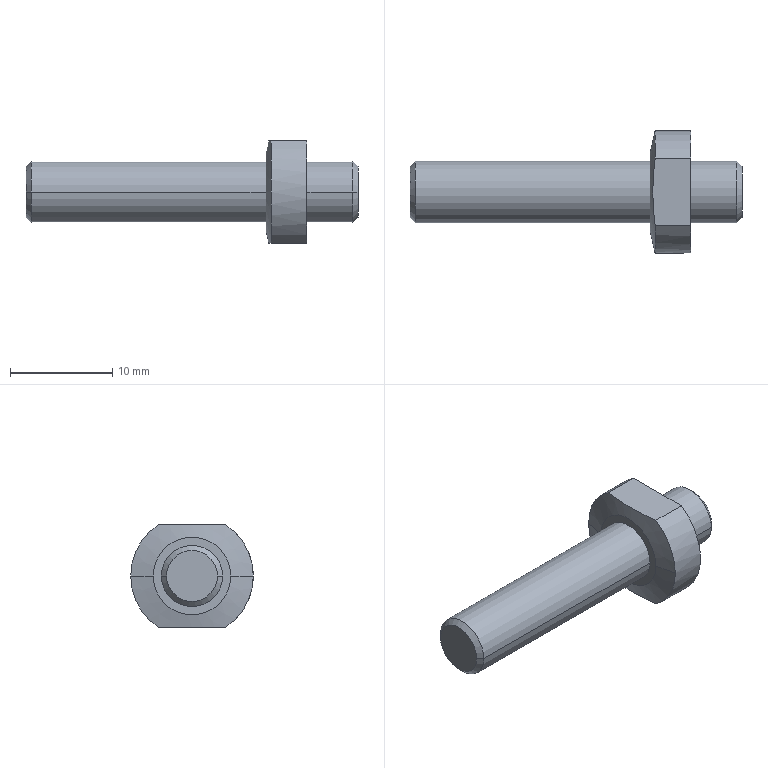Part | SolidWorks | features Chamfer 1, HoleWzd 1, ICE 1, Revolution 1 | 1 solid | 23 faces | box 32.5 x 12 x 10 mm | volume 1165 mm3 | cylinder 9 | cone 8 | plane 6 | commonest cylinder face diameters 6 x4 12 x3 2.5 x2
STEP:
#1=CARTESIAN_POINT('',(0.,-2.5,0.));
#2=VERTEX_POINT('',#1);
#3=CARTESIAN_POINT('',(0.,2.5,0.));
#4=VERTEX_POINT('',#3);
#5=CARTESIAN_POINT('',(0.,0.,0.));
#6=DIRECTION('',(-1.,0.,0.));
#7=DIRECTION('',(0.,-1.,0.));
#8=AXIS2_PLACEMENT_3D('',#5,#6,#7);
#9=CIRCLE('',#8,2.5);
#10=EDGE_CURVE('',#2,#4,#9,.T.);
#11=ORIENTED_EDGE('',*,*,#10,.F.);
#12=CARTESIAN_POINT('',(0.5,-3.,0.));
#13=VERTEX_POINT('',#12);
#14=CARTESIAN_POINT('',(0.5,-3.,0.));
#15=DIRECTION('',(0.7071,-0.7071,0.));
#16=VECTOR('',#15,1000.);
#17=LINE('',#14,#16);
#18=EDGE_CURVE('',#2,#13,#17,.T.);
#19=ORIENTED_EDGE('',*,*,#18,.T.);
#20=CARTESIAN_POINT('',(0.5,3.,0.));
#21=VERTEX_POINT('',#20);
#22=CARTESIAN_POINT('',(0.5,0.,0.));
#23=DIRECTION('',(1.,0.,0.));
#24=DIRECTION('',(0.,-1.,0.));
#25=AXIS2_PLACEMENT_3D('',#22,#23,#24);
#26=CIRCLE('',#25,3.);
#27=EDGE_CURVE('',#21,#13,#26,.T.);
#28=ORIENTED_EDGE('',*,*,#27,.F.);
#29=CARTESIAN_POINT('',(0.5,3.,0.));
#30=DIRECTION('',(0.7071,0.7071,0.));
#31=VECTOR('',#30,1000.);
#32=LINE('',#29,#31);
#33=EDGE_CURVE('',#4,#21,#32,.T.);
#34=ORIENTED_EDGE('',*,*,#33,.F.);
#35=EDGE_LOOP('',(#11,#19,#28,#34));
#36=FACE_OUTER_BOUND('',#35,.T.);
#37=CARTESIAN_POINT('',(0.5,0.,0.));
#38=DIRECTION('',(1.,0.,0.));
#39=DIRECTION('',(0.,1.,0.));
#40=AXIS2_PLACEMENT_3D('',#37,#38,#39);
#41=CONICAL_SURFACE('',#40,3.,0.7854);
#42=ADVANCED_FACE('',(#36),#41,.T.);
#43=CARTESIAN_POINT('',(32.5,2.5,0.));
#44=VERTEX_POINT('',#43);
#45=CARTESIAN_POINT('',(32.5,-2.5,0.));
#46=VERTEX_POINT('',#45);
#47=CARTESIAN_POINT('',(32.5,0.,0.));
#48=DIRECTION('',(1.,0.,0.));
#49=DIRECTION('',(0.,1.,0.));
#50=AXIS2_PLACEMENT_3D('',#47,#48,#49);
#51=CIRCLE('',#50,2.5);
#52=EDGE_CURVE('',#44,#46,#51,.T.);
#53=ORIENTED_EDGE('',*,*,#52,.F.);
#54=CARTESIAN_POINT('',(32.,3.,0.));
#55=VERTEX_POINT('',#54);
#56=CARTESIAN_POINT('',(32.5,2.5,0.));
#57=DIRECTION('',(-0.7071,0.7071,0.));
#58=VECTOR('',#57,1000.);
#59=LINE('',#56,#58);
#60=EDGE_CURVE('',#44,#55,#59,.T.);
#61=ORIENTED_EDGE('',*,*,#60,.T.);
#62=CARTESIAN_POINT('',(32.,-3.,0.));
#63=VERTEX_POINT('',#62);
#64=CARTESIAN_POINT('',(32.,0.,0.));
#65=DIRECTION('',(-1.,0.,0.));
#66=DIRECTION('',(0.,1.,0.));
#67=AXIS2_PLACEMENT_3D('',#64,#65,#66);
#68=CIRCLE('',#67,3.);
#69=EDGE_CURVE('',#63,#55,#68,.T.);
#70=ORIENTED_EDGE('',*,*,#69,.F.);
#71=CARTESIAN_POINT('',(32.5,-2.5,0.));
#72=DIRECTION('',(-0.7071,-0.7071,0.));
#73=VECTOR('',#72,1000.);
#74=LINE('',#71,#73);
#75=EDGE_CURVE('',#46,#63,#74,.T.);
#76=ORIENTED_EDGE('',*,*,#75,.F.);
#77=EDGE_LOOP('',(#53,#61,#70,#76));
#78=FACE_OUTER_BOUND('',#77,.T.);
#79=CARTESIAN_POINT('',(32.5,0.,0.));
#80=DIRECTION('',(-1.,0.,0.));
#81=DIRECTION('',(0.,-1.,0.));
#82=AXIS2_PLACEMENT_3D('',#79,#80,#81);
#83=CONICAL_SURFACE('',#82,2.5,0.7854);
#84=ADVANCED_FACE('',(#78),#83,.T.);
#85=CARTESIAN_POINT('',(25.,0.,1.25));
#86=VERTEX_POINT('',#85);
#87=CARTESIAN_POINT('',(25.,0.,-1.25));
#88=VERTEX_POINT('',#87);
#89=CARTESIAN_POINT('',(25.,0.,0.));
#90=DIRECTION('',(1.,0.,0.));
#91=DIRECTION('',(0.,0.,-1.));
#92=AXIS2_PLACEMENT_3D('',#89,#90,#91);
#93=CIRCLE('',#92,1.25);
#94=EDGE_CURVE('',#86,#88,#93,.T.);
#95=ORIENTED_EDGE('',*,*,#94,.F.);
#96=CARTESIAN_POINT('',(32.5,0.,1.25));
#97=VERTEX_POINT('',#96);
#98=CARTESIAN_POINT('',(32.5,0.,1.25));
#99=DIRECTION('',(1.,0.,0.));
#100=VECTOR('',#99,1000.);
#101=LINE('',#98,#100);
#102=EDGE_CURVE('',#86,#97,#101,.T.);
#103=ORIENTED_EDGE('',*,*,#102,.T.);
#104=CARTESIAN_POINT('',(32.5,0.,-1.25));
#105=VERTEX_POINT('',#104);
#106=CARTESIAN_POINT('',(32.5,0.,0.));
#107=DIRECTION('',(1.,0.,0.));
#108=DIRECTION('',(0.,0.,-1.));
#109=AXIS2_PLACEMENT_3D('',#106,#107,#108);
#110=CIRCLE('',#109,1.25);
#111=EDGE_CURVE('',#97,#105,#110,.T.);
#112=ORIENTED_EDGE('',*,*,#111,.T.);
#113=CARTESIAN_POINT('',(32.5,0.,-1.25));
#114=DIRECTION('',(1.,0.,0.));
#115=VECTOR('',#114,1000.);
#116=LINE('',#113,#115);
#117=EDGE_CURVE('',#88,#105,#116,.T.);
#118=ORIENTED_EDGE('',*,*,#117,.F.);
#119=EDGE_LOOP('',(#95,#103,#112,#118));
#120=FACE_OUTER_BOUND('',#119,.T.);
#121=CARTESIAN_POINT('',(32.5,0.,0.));
#122=DIRECTION('',(1.,0.,0.));
#123=DIRECTION('',(0.,0.,-1.));
#124=AXIS2_PLACEMENT_3D('',#121,#122,#123);
#125=CYLINDRICAL_SURFACE('',#124,1.25);
#126=ADVANCED_FACE('',(#120),#125,.F.);
#127=CARTESIAN_POINT('',(24.249,0.,0.));
#128=VERTEX_POINT('',#127);
#129=CARTESIAN_POINT('',(25.,0.,-1.25));
#130=DIRECTION('',(0.515,0.,-0.8572));
#131=VECTOR('',#130,1000.);
#132=LINE('',#129,#131);
#133=EDGE_CURVE('',#128,#88,#132,.T.);
#134=ORIENTED_EDGE('',*,*,#133,.F.);
#135=CARTESIAN_POINT('',(25.,0.,1.25));
#136=DIRECTION('',(0.515,0.,0.8572));
#137=VECTOR('',#136,1000.);
#138=LINE('',#135,#137);
#139=EDGE_CURVE('',#128,#86,#138,.T.);
#140=ORIENTED_EDGE('',*,*,#139,.T.);
#141=ORIENTED_EDGE('',*,*,#94,.T.);
#142=EDGE_LOOP('',(#134,#140,#141));
#143=FACE_OUTER_BOUND('',#142,.T.);
#144=CARTESIAN_POINT('',(25.,0.,0.));
#145=DIRECTION('',(1.,0.,0.));
#146=DIRECTION('',(0.,0.,-1.));
#147=AXIS2_PLACEMENT_3D('',#144,#145,#146);
#148=CONICAL_SURFACE('',#147,1.25,1.03);
#149=ADVANCED_FACE('',(#143),#148,.F.);
#150=CARTESIAN_POINT('',(27.5,3.,0.));
#151=VERTEX_POINT('',#150);
#152=CARTESIAN_POINT('',(27.5,-3.,0.));
#153=VERTEX_POINT('',#152);
#154=CARTESIAN_POINT('',(27.5,0.,0.));
#155=DIRECTION('',(1.,0.,0.));
#156=DIRECTION('',(0.,1.,0.));
#157=AXIS2_PLACEMENT_3D('',#154,#155,#156);
#158=CIRCLE('',#157,3.);
#159=EDGE_CURVE('',#151,#153,#158,.T.);
#160=ORIENTED_EDGE('',*,*,#159,.T.);
#161=CARTESIAN_POINT('',(32.5,-3.,0.));
#162=DIRECTION('',(1.,0.,0.));
#163=VECTOR('',#162,1000.);
#164=LINE('',#161,#163);
#165=EDGE_CURVE('',#153,#63,#164,.T.);
#166=ORIENTED_EDGE('',*,*,#165,.T.);
#167=ORIENTED_EDGE('',*,*,#69,.T.);
#168=CARTESIAN_POINT('',(32.5,3.,0.));
#169=DIRECTION('',(1.,0.,0.));
#170=VECTOR('',#169,1000.);
#171=LINE('',#168,#170);
#172=EDGE_CURVE('',#151,#55,#171,.T.);
#173=ORIENTED_EDGE('',*,*,#172,.F.);
#174=EDGE_LOOP('',(#160,#166,#167,#173));
#175=FACE_OUTER_BOUND('',#174,.T.);
#176=CARTESIAN_POINT('',(32.5,0.,0.));
#177=DIRECTION('',(1.,0.,0.));
#178=DIRECTION('',(0.,1.,0.));
#179=AXIS2_PLACEMENT_3D('',#176,#177,#178);
#180=CYLINDRICAL_SURFACE('',#179,3.);
#181=ADVANCED_FACE('',(#175),#180,.T.);
#182=ORIENTED_EDGE('',*,*,#27,.T.);
#183=CARTESIAN_POINT('',(23.5,-3.,0.));
#184=VERTEX_POINT('',#183);
#185=CARTESIAN_POINT('',(32.5,-3.,0.));
#186=DIRECTION('',(1.,0.,0.));
#187=VECTOR('',#186,1000.);
#188=LINE('',#185,#187);
#189=EDGE_CURVE('',#13,#184,#188,.T.);
#190=ORIENTED_EDGE('',*,*,#189,.T.);
#191=CARTESIAN_POINT('',(23.5,3.,0.));
#192=VERTEX_POINT('',#191);
#193=CARTESIAN_POINT('',(23.5,0.,0.));
#194=DIRECTION('',(1.,0.,0.));
#195=DIRECTION('',(0.,1.,0.));
#196=AXIS2_PLACEMENT_3D('',#193,#194,#195);
#197=CIRCLE('',#196,3.);
#198=EDGE_CURVE('',#192,#184,#197,.T.);
#199=ORIENTED_EDGE('',*,*,#198,.F.);
#200=CARTESIAN_POINT('',(32.5,3.,0.));
#201=DIRECTION('',(1.,0.,0.));
#202=VECTOR('',#201,1000.);
#203=LINE('',#200,#202);
#204=EDGE_CURVE('',#21,#192,#203,.T.);
#205=ORIENTED_EDGE('',*,*,#204,.F.);
#206=EDGE_LOOP('',(#182,#190,#199,#205));
#207=FACE_OUTER_BOUND('',#206,.T.);
#208=CARTESIAN_POINT('',(32.5,0.,0.));
#209=DIRECTION('',(1.,0.,0.));
#210=DIRECTION('',(0.,1.,0.));
#211=AXIS2_PLACEMENT_3D('',#208,#209,#210);
#212=CYLINDRICAL_SURFACE('',#211,3.);
#213=ADVANCED_FACE('',(#207),#212,.T.);
#214=CARTESIAN_POINT('',(24.,3.317,-5.));
#215=VERTEX_POINT('',#214);
#216=CARTESIAN_POINT('',(24.,6.,0.));
#217=VERTEX_POINT('',#216);
#218=CARTESIAN_POINT('',(24.,0.,0.));
#219=DIRECTION('',(1.,0.,0.));
#220=DIRECTION('',(0.,1.,0.));
#221=AXIS2_PLACEMENT_3D('',#218,#219,#220);
#222=CIRCLE('',#221,6.);
#223=EDGE_CURVE('',#215,#217,#222,.T.);
#224=ORIENTED_EDGE('',*,*,#223,.T.);
#225=CARTESIAN_POINT('',(27.5,6.,0.));
#226=VERTEX_POINT('',#225);
#227=CARTESIAN_POINT('',(32.5,6.,0.));
#228=DIRECTION('',(1.,0.,0.));
#229=VECTOR('',#228,1000.);
#230=LINE('',#227,#229);
#231=EDGE_CURVE('',#217,#226,#230,.T.);
#232=ORIENTED_EDGE('',*,*,#231,.T.);
#233=CARTESIAN_POINT('',(27.5,3.317,-5.));
#234=VERTEX_POINT('',#233);
#235=CARTESIAN_POINT('',(27.5,0.,0.));
#236=DIRECTION('',(1.,0.,0.));
#237=DIRECTION('',(0.,1.,0.));
#238=AXIS2_PLACEMENT_3D('',#235,#236,#237);
#239=CIRCLE('',#238,6.);
#240=EDGE_CURVE('',#234,#226,#239,.T.);
#241=ORIENTED_EDGE('',*,*,#240,.F.);
#242=CARTESIAN_POINT('',(32.5,3.317,-5.));
#243=DIRECTION('',(-1.,0.,0.));
#244=VECTOR('',#243,1000.);
#245=LINE('',#242,#244);
#246=EDGE_CURVE('',#234,#215,#245,.T.);
#247=ORIENTED_EDGE('',*,*,#246,.T.);
#248=EDGE_LOOP('',(#224,#232,#241,#247));
#249=FACE_OUTER_BOUND('',#248,.T.);
#250=CARTESIAN_POINT('',(32.5,0.,0.));
#251=DIRECTION('',(1.,0.,0.));
#252=DIRECTION('',(0.,1.,0.));
#253=AXIS2_PLACEMENT_3D('',#250,#251,#252);
#254=CYLINDRICAL_SURFACE('',#253,6.);
#255=ADVANCED_FACE('',(#249),#254,.T.);
#256=CARTESIAN_POINT('',(23.5,3.8,0.));
#257=VERTEX_POINT('',#256);
#258=CARTESIAN_POINT('',(23.5,-3.8,0.));
#259=VERTEX_POINT('',#258);
#260=CARTESIAN_POINT('',(23.5,0.,0.));
#261=DIRECTION('',(1.,0.,0.));
#262=DIRECTION('',(0.,1.,0.));
#263=AXIS2_PLACEMENT_3D('',#260,#261,#262);
#264=CIRCLE('',#263,3.8);
#265=EDGE_CURVE('',#257,#259,#264,.T.);
#266=ORIENTED_EDGE('',*,*,#265,.T.);
#267=CARTESIAN_POINT('',(24.,-6.,0.));
#268=VERTEX_POINT('',#267);
#269=CARTESIAN_POINT('',(24.,-6.,0.));
#270=DIRECTION('',(0.2216,-0.9751,0.));
#271=VECTOR('',#270,1000.);
#272=LINE('',#269,#271);
#273=EDGE_CURVE('',#259,#268,#272,.T.);
#274=ORIENTED_EDGE('',*,*,#273,.T.);
#275=CARTESIAN_POINT('',(24.,-3.317,5.));
#276=VERTEX_POINT('',#275);
#277=CARTESIAN_POINT('',(24.,0.,0.));
#278=DIRECTION('',(1.,0.,0.));
#279=DIRECTION('',(0.,1.,0.));
#280=AXIS2_PLACEMENT_3D('',#277,#278,#279);
#281=CIRCLE('',#280,6.);
#282=EDGE_CURVE('',#276,#268,#281,.T.);
#283=ORIENTED_EDGE('',*,*,#282,.F.);
#284=CARTESIAN_POINT('',(24.,3.317,5.));
#285=VERTEX_POINT('',#284);
#286=CARTESIAN_POINT('',(24.,-3.317,5.));
#287=CARTESIAN_POINT('',(23.861,-2.214,5.));
#288=CARTESIAN_POINT('',(23.773,-1.11,5.));
#289=CARTESIAN_POINT('',(23.773,0.549,5.));
#290=CARTESIAN_POINT('',(23.794,1.102,5.));
#291=CARTESIAN_POINT('',(23.873,2.21,5.));
#292=CARTESIAN_POINT('',(23.931,2.765,5.));
#293=CARTESIAN_POINT('',(24.,3.317,5.));
#294=B_SPLINE_CURVE_WITH_KNOTS('',3,(#286,#287,#288,#289,#290,#291,#292,#293),.UNSPECIFIED.,.F.,.F.,(4,2,2,4),(0.006705,0.01004,0.01171,0.01338),.UNSPECIFIED.);
#295=EDGE_CURVE('',#276,#285,#294,.T.);
#296=ORIENTED_EDGE('',*,*,#295,.T.);
#297=CARTESIAN_POINT('',(24.,0.,0.));
#298=DIRECTION('',(1.,0.,0.));
#299=DIRECTION('',(0.,1.,0.));
#300=AXIS2_PLACEMENT_3D('',#297,#298,#299);
#301=CIRCLE('',#300,6.);
#302=EDGE_CURVE('',#217,#285,#301,.T.);
#303=ORIENTED_EDGE('',*,*,#302,.F.);
#304=CARTESIAN_POINT('',(24.,6.,0.));
#305=DIRECTION('',(0.2216,0.9751,0.));
#306=VECTOR('',#305,1000.);
#307=LINE('',#304,#306);
#308=EDGE_CURVE('',#257,#217,#307,.T.);
#309=ORIENTED_EDGE('',*,*,#308,.F.);
#310=EDGE_LOOP('',(#266,#274,#283,#296,#303,#309));
#311=FACE_OUTER_BOUND('',#310,.T.);
#312=CARTESIAN_POINT('',(24.,0.,0.));
#313=DIRECTION('',(1.,0.,0.));
#314=DIRECTION('',(0.,1.,0.));
#315=AXIS2_PLACEMENT_3D('',#312,#313,#314);
#316=CONICAL_SURFACE('',#315,6.,1.347);
#317=ADVANCED_FACE('',(#311),#316,.T.);
#318=ORIENTED_EDGE('',*,*,#273,.F.);
#319=CARTESIAN_POINT('',(23.5,0.,0.));
#320=DIRECTION('',(1.,0.,0.));
#321=DIRECTION('',(0.,1.,0.));
#322=AXIS2_PLACEMENT_3D('',#319,#320,#321);
#323=CIRCLE('',#322,3.8);
#324=EDGE_CURVE('',#259,#257,#323,.T.);
#325=ORIENTED_EDGE('',*,*,#324,.T.);
#326=ORIENTED_EDGE('',*,*,#308,.T.);
#327=ORIENTED_EDGE('',*,*,#223,.F.);
#328=CARTESIAN_POINT('',(24.,-3.317,-5.));
#329=VERTEX_POINT('',#328);
#330=CARTESIAN_POINT('',(24.,3.317,-5.));
#331=CARTESIAN_POINT('',(23.931,2.765,-5.));
#332=CARTESIAN_POINT('',(23.873,2.21,-5.));
#333=CARTESIAN_POINT('',(23.794,1.102,-5.));
#334=CARTESIAN_POINT('',(23.773,0.549,-5.));
#335=CARTESIAN_POINT('',(23.773,-1.11,-5.));
#336=CARTESIAN_POINT('',(23.861,-2.214,-5.));
#337=CARTESIAN_POINT('',(24.,-3.317,-5.));
#338=B_SPLINE_CURVE_WITH_KNOTS('',3,(#330,#331,#332,#333,#334,#335,#336,#337),.UNSPECIFIED.,.F.,.F.,(4,2,2,4),(0.02106,0.02273,0.02439,0.02772),.UNSPECIFIED.);
#339=EDGE_CURVE('',#215,#329,#338,.T.);
#340=ORIENTED_EDGE('',*,*,#339,.T.);
#341=CARTESIAN_POINT('',(24.,0.,0.));
#342=DIRECTION('',(1.,0.,0.));
#343=DIRECTION('',(0.,1.,0.));
#344=AXIS2_PLACEMENT_3D('',#341,#342,#343);
#345=CIRCLE('',#344,6.);
#346=EDGE_CURVE('',#268,#329,#345,.T.);
#347=ORIENTED_EDGE('',*,*,#346,.F.);
#348=EDGE_LOOP('',(#318,#325,#326,#327,#340,#347));
#349=FACE_OUTER_BOUND('',#348,.T.);
#350=CARTESIAN_POINT('',(24.,0.,0.));
#351=DIRECTION('',(1.,0.,0.));
#352=DIRECTION('',(0.,1.,0.));
#353=AXIS2_PLACEMENT_3D('',#350,#351,#352);
#354=CONICAL_SURFACE('',#353,6.,1.347);
#355=ADVANCED_FACE('',(#349),#354,.T.);
#356=CARTESIAN_POINT('',(27.5,-3.317,5.));
#357=VERTEX_POINT('',#356);
#358=CARTESIAN_POINT('',(27.5,-3.317,-5.));
#359=VERTEX_POINT('',#358);
#360=CARTESIAN_POINT('',(27.5,0.,0.));
#361=DIRECTION('',(1.,0.,0.));
#362=DIRECTION('',(0.,1.,0.));
#363=AXIS2_PLACEMENT_3D('',#360,#361,#362);
#364=CIRCLE('',#363,6.);
#365=EDGE_CURVE('',#357,#359,#364,.T.);
#366=ORIENTED_EDGE('',*,*,#365,.F.);
#367=CARTESIAN_POINT('',(32.5,-3.317,5.));
#368=DIRECTION('',(-1.,0.,0.));
#369=VECTOR('',#368,1000.);
#370=LINE('',#367,#369);
#371=EDGE_CURVE('',#357,#276,#370,.T.);
#372=ORIENTED_EDGE('',*,*,#371,.T.);
#373=ORIENTED_EDGE('',*,*,#282,.T.);
#374=ORIENTED_EDGE('',*,*,#346,.T.);
#375=CARTESIAN_POINT('',(32.5,-3.317,-5.));
#376=DIRECTION('',(1.,0.,0.));
#377=VECTOR('',#376,1000.);
#378=LINE('',#375,#377);
#379=EDGE_CURVE('',#329,#359,#378,.T.);
#380=ORIENTED_EDGE('',*,*,#379,.T.);
#381=EDGE_LOOP('',(#366,#372,#373,#374,#380));
#382=FACE_OUTER_BOUND('',#381,.T.);
#383=CARTESIAN_POINT('',(32.5,0.,0.));
#384=DIRECTION('',(1.,0.,0.));
#385=DIRECTION('',(0.,1.,0.));
#386=AXIS2_PLACEMENT_3D('',#383,#384,#385);
#387=CYLINDRICAL_SURFACE('',#386,6.);
#388=ADVANCED_FACE('',(#382),#387,.T.);
#389=ORIENTED_EDGE('',*,*,#231,.F.);
#390=ORIENTED_EDGE('',*,*,#302,.T.);
#391=CARTESIAN_POINT('',(27.5,3.317,5.));
#392=VERTEX_POINT('',#391);
#393=CARTESIAN_POINT('',(32.5,3.317,5.));
#394=DIRECTION('',(1.,0.,0.));
#395=VECTOR('',#394,1000.);
#396=LINE('',#393,#395);
#397=EDGE_CURVE('',#285,#392,#396,.T.);
#398=ORIENTED_EDGE('',*,*,#397,.T.);
#399=CARTESIAN_POINT('',(27.5,0.,0.));
#400=DIRECTION('',(1.,0.,0.));
#401=DIRECTION('',(0.,1.,0.));
#402=AXIS2_PLACEMENT_3D('',#399,#400,#401);
#403=CIRCLE('',#402,6.);
#404=EDGE_CURVE('',#226,#392,#403,.T.);
#405=ORIENTED_EDGE('',*,*,#404,.F.);
#406=EDGE_LOOP('',(#389,#390,#398,#405));
#407=FACE_OUTER_BOUND('',#406,.T.);
#408=CARTESIAN_POINT('',(32.5,0.,0.));
#409=DIRECTION('',(1.,0.,0.));
#410=DIRECTION('',(0.,1.,0.));
#411=AXIS2_PLACEMENT_3D('',#408,#409,#410);
#412=CYLINDRICAL_SURFACE('',#411,6.);
#413=ADVANCED_FACE('',(#407),#412,.T.);
#414=ORIENTED_EDGE('',*,*,#159,.F.);
#415=CARTESIAN_POINT('',(27.5,0.,0.));
#416=DIRECTION('',(1.,0.,0.));
#417=DIRECTION('',(0.,1.,0.));
#418=AXIS2_PLACEMENT_3D('',#415,#416,#417);
#419=CIRCLE('',#418,3.);
#420=EDGE_CURVE('',#153,#151,#419,.T.);
#421=ORIENTED_EDGE('',*,*,#420,.F.);
#422=EDGE_LOOP('',(#414,#421));
#423=FACE_BOUND('',#422,.T.);
#424=ORIENTED_EDGE('',*,*,#240,.T.);
#425=ORIENTED_EDGE('',*,*,#404,.T.);
#426=CARTESIAN_POINT('',(27.5,6.,5.));
#427=DIRECTION('',(0.,-1.,0.));
#428=VECTOR('',#427,1000.);
#429=LINE('',#426,#428);
#430=EDGE_CURVE('',#392,#357,#429,.T.);
#431=ORIENTED_EDGE('',*,*,#430,.T.);
#432=ORIENTED_EDGE('',*,*,#365,.T.);
#433=CARTESIAN_POINT('',(27.5,6.,-5.));
#434=DIRECTION('',(0.,1.,0.));
#435=VECTOR('',#434,1000.);
#436=LINE('',#433,#435);
#437=EDGE_CURVE('',#359,#234,#436,.T.);
#438=ORIENTED_EDGE('',*,*,#437,.T.);
#439=EDGE_LOOP('',(#424,#425,#431,#432,#438));
#440=FACE_OUTER_BOUND('',#439,.T.);
#441=CARTESIAN_POINT('',(27.5,6.,0.));
#442=DIRECTION('',(1.,0.,0.));
#443=DIRECTION('',(0.,1.,0.));
#444=AXIS2_PLACEMENT_3D('',#441,#442,#443);
#445=PLANE('',#444);
#446=ADVANCED_FACE('',(#423,#440),#445,.T.);
#447=CARTESIAN_POINT('',(0.,0.,0.));
#448=DIRECTION('',(-1.,0.,0.));
#449=DIRECTION('',(0.,-1.,0.));
#450=AXIS2_PLACEMENT_3D('',#447,#448,#449);
#451=CIRCLE('',#450,2.5);
#452=EDGE_CURVE('',#4,#2,#451,.T.);
#453=ORIENTED_EDGE('',*,*,#452,.T.);
#454=ORIENTED_EDGE('',*,*,#10,.T.);
#455=EDGE_LOOP('',(#453,#454));
#456=FACE_OUTER_BOUND('',#455,.T.);
#457=CARTESIAN_POINT('',(0.,0.,0.));
#458=DIRECTION('',(-1.,0.,0.));
#459=DIRECTION('',(0.,-1.,0.));
#460=AXIS2_PLACEMENT_3D('',#457,#458,#459);
#461=PLANE('',#460);
#462=ADVANCED_FACE('',(#456),#461,.T.);
#463=ORIENTED_EDGE('',*,*,#189,.F.);
#464=CARTESIAN_POINT('',(0.5,0.,0.));
#465=DIRECTION('',(1.,0.,0.));
#466=DIRECTION('',(0.,-1.,0.));
#467=AXIS2_PLACEMENT_3D('',#464,#465,#466);
#468=CIRCLE('',#467,3.);
#469=EDGE_CURVE('',#13,#21,#468,.T.);
#470=ORIENTED_EDGE('',*,*,#469,.T.);
#471=ORIENTED_EDGE('',*,*,#204,.T.);
#472=CARTESIAN_POINT('',(23.5,0.,0.));
#473=DIRECTION('',(1.,0.,0.));
#474=DIRECTION('',(0.,1.,0.));
#475=AXIS2_PLACEMENT_3D('',#472,#473,#474);
#476=CIRCLE('',#475,3.);
#477=EDGE_CURVE('',#184,#192,#476,.T.);
#478=ORIENTED_EDGE('',*,*,#477,.F.);
#479=EDGE_LOOP('',(#463,#470,#471,#478));
#480=FACE_OUTER_BOUND('',#479,.T.);
#481=CARTESIAN_POINT('',(32.5,0.,0.));
#482=DIRECTION('',(1.,0.,0.));
#483=DIRECTION('',(0.,1.,0.));
#484=AXIS2_PLACEMENT_3D('',#481,#482,#483);
#485=CYLINDRICAL_SURFACE('',#484,3.);
#486=ADVANCED_FACE('',(#480),#485,.T.);
#487=ORIENTED_EDGE('',*,*,#198,.T.);
#488=ORIENTED_EDGE('',*,*,#477,.T.);
#489=EDGE_LOOP('',(#487,#488));
#490=FACE_BOUND('',#489,.T.);
#491=ORIENTED_EDGE('',*,*,#265,.F.);
#492=ORIENTED_EDGE('',*,*,#324,.F.);
#493=EDGE_LOOP('',(#491,#492));
#494=FACE_OUTER_BOUND('',#493,.T.);
#495=CARTESIAN_POINT('',(23.5,3.8,0.));
#496=DIRECTION('',(-1.,0.,0.));
#497=DIRECTION('',(0.,-1.,0.));
#498=AXIS2_PLACEMENT_3D('',#495,#496,#497);
#499=PLANE('',#498);
#500=ADVANCED_FACE('',(#490,#494),#499,.T.);
#501=ORIENTED_EDGE('',*,*,#165,.F.);
#502=ORIENTED_EDGE('',*,*,#420,.T.);
#503=ORIENTED_EDGE('',*,*,#172,.T.);
#504=CARTESIAN_POINT('',(32.,0.,0.));
#505=DIRECTION('',(-1.,0.,0.));
#506=DIRECTION('',(0.,1.,0.));
#507=AXIS2_PLACEMENT_3D('',#504,#505,#506);
#508=CIRCLE('',#507,3.);
#509=EDGE_CURVE('',#55,#63,#508,.T.);
#510=ORIENTED_EDGE('',*,*,#509,.T.);
#511=EDGE_LOOP('',(#501,#502,#503,#510));
#512=FACE_OUTER_BOUND('',#511,.T.);
#513=CARTESIAN_POINT('',(32.5,0.,0.));
#514=DIRECTION('',(1.,0.,0.));
#515=DIRECTION('',(0.,1.,0.));
#516=AXIS2_PLACEMENT_3D('',#513,#514,#515);
#517=CYLINDRICAL_SURFACE('',#516,3.);
#518=ADVANCED_FACE('',(#512),#517,.T.);
#519=CARTESIAN_POINT('',(32.5,0.,0.));
#520=DIRECTION('',(1.,0.,0.));
#521=DIRECTION('',(0.,1.,0.));
#522=AXIS2_PLACEMENT_3D('',#519,#520,#521);
#523=CIRCLE('',#522,2.5);
#524=EDGE_CURVE('',#46,#44,#523,.T.);
#525=ORIENTED_EDGE('',*,*,#524,.T.);
#526=ORIENTED_EDGE('',*,*,#52,.T.);
#527=EDGE_LOOP('',(#525,#526));
#528=FACE_OUTER_BOUND('',#527,.T.);
#529=CARTESIAN_POINT('',(32.5,0.,0.));
#530=DIRECTION('',(1.,0.,0.));
#531=DIRECTION('',(0.,0.,-1.));
#532=AXIS2_PLACEMENT_3D('',#529,#530,#531);
#533=CIRCLE('',#532,1.25);
#534=EDGE_CURVE('',#105,#97,#533,.T.);
#535=ORIENTED_EDGE('',*,*,#534,.F.);
#536=ORIENTED_EDGE('',*,*,#111,.F.);
#537=EDGE_LOOP('',(#535,#536));
#538=FACE_BOUND('',#537,.T.);
#539=CARTESIAN_POINT('',(32.5,3.,0.));
#540=DIRECTION('',(1.,0.,0.));
#541=DIRECTION('',(0.,1.,0.));
#542=AXIS2_PLACEMENT_3D('',#539,#540,#541);
#543=PLANE('',#542);
#544=ADVANCED_FACE('',(#528,#538),#543,.T.);
#545=ORIENTED_EDGE('',*,*,#437,.F.);
#546=ORIENTED_EDGE('',*,*,#379,.F.);
#547=ORIENTED_EDGE('',*,*,#339,.F.);
#548=ORIENTED_EDGE('',*,*,#246,.F.);
#549=EDGE_LOOP('',(#545,#546,#547,#548));
#550=FACE_OUTER_BOUND('',#549,.T.);
#551=CARTESIAN_POINT('',(0.,-12.284,-5.));
#552=DIRECTION('',(0.,0.,-1.));
#553=DIRECTION('',(-1.,0.,0.));
#554=AXIS2_PLACEMENT_3D('',#551,#552,#553);
#555=PLANE('',#554);
#556=ADVANCED_FACE('',(#550),#555,.T.);
#557=ORIENTED_EDGE('',*,*,#430,.F.);
#558=ORIENTED_EDGE('',*,*,#397,.F.);
#559=ORIENTED_EDGE('',*,*,#295,.F.);
#560=ORIENTED_EDGE('',*,*,#371,.F.);
#561=EDGE_LOOP('',(#557,#558,#559,#560));
#562=FACE_OUTER_BOUND('',#561,.T.);
#563=CARTESIAN_POINT('',(0.,-12.284,5.));
#564=DIRECTION('',(0.,0.,1.));
#565=DIRECTION('',(1.,0.,0.));
#566=AXIS2_PLACEMENT_3D('',#563,#564,#565);
#567=PLANE('',#566);
#568=ADVANCED_FACE('',(#562),#567,.T.);
#569=ORIENTED_EDGE('',*,*,#139,.F.);
#570=ORIENTED_EDGE('',*,*,#133,.T.);
#571=CARTESIAN_POINT('',(25.,0.,0.));
#572=DIRECTION('',(1.,0.,0.));
#573=DIRECTION('',(0.,0.,-1.));
#574=AXIS2_PLACEMENT_3D('',#571,#572,#573);
#575=CIRCLE('',#574,1.25);
#576=EDGE_CURVE('',#88,#86,#575,.T.);
#577=ORIENTED_EDGE('',*,*,#576,.T.);
#578=EDGE_LOOP('',(#569,#570,#577));
#579=FACE_OUTER_BOUND('',#578,.T.);
#580=CARTESIAN_POINT('',(25.,0.,0.));
#581=DIRECTION('',(1.,0.,0.));
#582=DIRECTION('',(0.,0.,-1.));
#583=AXIS2_PLACEMENT_3D('',#580,#581,#582);
#584=CONICAL_SURFACE('',#583,1.25,1.03);
#585=ADVANCED_FACE('',(#579),#584,.F.);
#586=ORIENTED_EDGE('',*,*,#102,.F.);
#587=ORIENTED_EDGE('',*,*,#576,.F.);
#588=ORIENTED_EDGE('',*,*,#117,.T.);
#589=ORIENTED_EDGE('',*,*,#534,.T.);
#590=EDGE_LOOP('',(#586,#587,#588,#589));
#591=FACE_OUTER_BOUND('',#590,.T.);
#592=CARTESIAN_POINT('',(32.5,0.,0.));
#593=DIRECTION('',(1.,0.,0.));
#594=DIRECTION('',(0.,0.,-1.));
#595=AXIS2_PLACEMENT_3D('',#592,#593,#594);
#596=CYLINDRICAL_SURFACE('',#595,1.25);
#597=ADVANCED_FACE('',(#591),#596,.F.);
#598=ORIENTED_EDGE('',*,*,#60,.F.);
#599=ORIENTED_EDGE('',*,*,#524,.F.);
#600=ORIENTED_EDGE('',*,*,#75,.T.);
#601=ORIENTED_EDGE('',*,*,#509,.F.);
#602=EDGE_LOOP('',(#598,#599,#600,#601));
#603=FACE_OUTER_BOUND('',#602,.T.);
#604=CARTESIAN_POINT('',(32.5,0.,0.));
#605=DIRECTION('',(-1.,0.,0.));
#606=DIRECTION('',(0.,-1.,0.));
#607=AXIS2_PLACEMENT_3D('',#604,#605,#606);
#608=CONICAL_SURFACE('',#607,2.5,0.7854);
#609=ADVANCED_FACE('',(#603),#608,.T.);
#610=ORIENTED_EDGE('',*,*,#18,.F.);
#611=ORIENTED_EDGE('',*,*,#452,.F.);
#612=ORIENTED_EDGE('',*,*,#33,.T.);
#613=ORIENTED_EDGE('',*,*,#469,.F.);
#614=EDGE_LOOP('',(#610,#611,#612,#613));
#615=FACE_OUTER_BOUND('',#614,.T.);
#616=CARTESIAN_POINT('',(0.5,0.,0.));
#617=DIRECTION('',(1.,0.,0.));
#618=DIRECTION('',(0.,1.,0.));
#619=AXIS2_PLACEMENT_3D('',#616,#617,#618);
#620=CONICAL_SURFACE('',#619,3.,0.7854);
#621=ADVANCED_FACE('',(#615),#620,.T.);
#622=CLOSED_SHELL('',(#42,#84,#126,#149,#181,#213,#255,#317,#355,#388,#413,#446,#462,#486,#500,#518,#544,#556,#568,#585,#597,#609,#621));
#623=MANIFOLD_SOLID_BREP('',#622);
#624=CARTESIAN_POINT('',(0.,0.,0.));
#625=DIRECTION('',(0.,0.,1.));
#626=DIRECTION('',(1.,0.,0.));
#627=AXIS2_PLACEMENT_3D('',#624,#625,#626);
#628=(LENGTH_UNIT()NAMED_UNIT(*)SI_UNIT(.MILLI.,.METRE.));
#629=UNCERTAINTY_MEASURE_WITH_UNIT(LENGTH_MEASURE(0.00001),#628,'','');
#630=(NAMED_UNIT(*)PLANE_ANGLE_UNIT()SI_UNIT($,.RADIAN.));
#631=(NAMED_UNIT(*)SI_UNIT($,.STERADIAN.)SOLID_ANGLE_UNIT());
#632=(GEOMETRIC_REPRESENTATION_CONTEXT(3)GLOBAL_UNCERTAINTY_ASSIGNED_CONTEXT((#629))GLOBAL_UNIT_ASSIGNED_CONTEXT((#628,#630,#631))REPRESENTATION_CONTEXT('',''));
#633=ADVANCED_BREP_SHAPE_REPRESENTATION('',(#623,#627),#632);